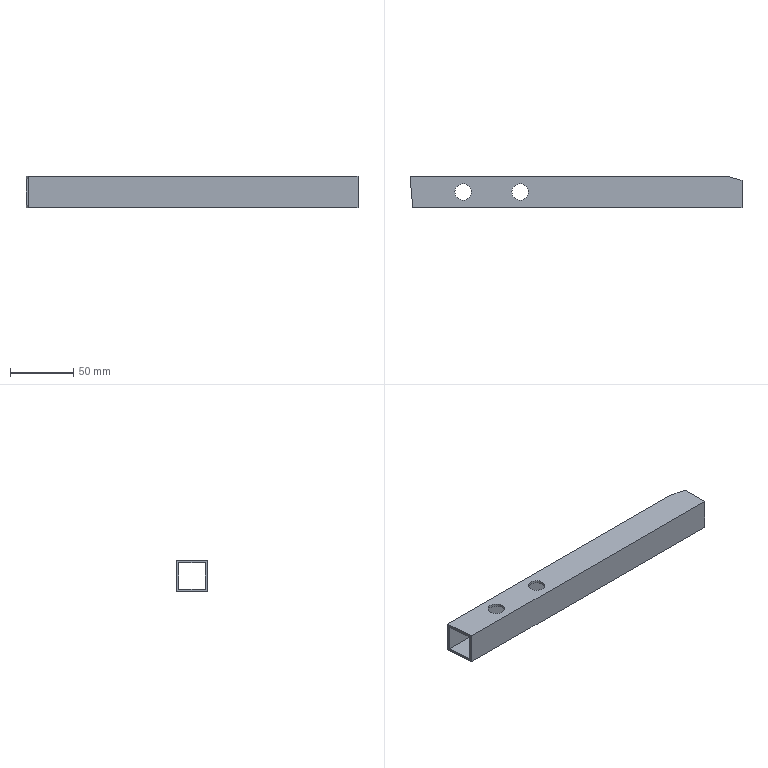Part | NX | features solid 2 | 1 solid | 15 faces | box 261.968 x 25 x 25 mm | volume 46481 mm3 | plane 11 | cylinder 4 | commonest cylinder face diameters 13 x4
STEP:
#1=CARTESIAN_POINT('',(636.5,-100.,-30.));
#2=VERTEX_POINT('',#1);
#3=CARTESIAN_POINT('',(630.,-100.,-30.));
#4=DIRECTION('',(0.,0.,1.));
#5=DIRECTION('',(1.,0.,0.));
#6=AXIS2_PLACEMENT_3D('',#3,#4,#5);
#7=CIRCLE('',#6,6.5);
#8=EDGE_CURVE('',#2,#2,#7,.T.);
#9=ORIENTED_EDGE('',*,*,#8,.F.);
#10=EDGE_LOOP('',(#9));
#11=FACE_BOUND('',#10,.T.);
#12=CARTESIAN_POINT('',(850.,-90.878,-30.));
#13=VERTEX_POINT('',#12);
#14=CARTESIAN_POINT('',(837.392,-87.5,-30.));
#15=VERTEX_POINT('',#14);
#16=CARTESIAN_POINT('',(699.873,-50.652,-30.));
#17=DIRECTION('',(0.9659,-0.2588,0.));
#18=VECTOR('',#17,1000.);
#19=LINE('',#16,#18);
#20=EDGE_CURVE('',#13,#15,#19,.F.);
#21=ORIENTED_EDGE('',*,*,#20,.T.);
#22=CARTESIAN_POINT('',(588.032,-87.5,-30.));
#23=VERTEX_POINT('',#22);
#24=CARTESIAN_POINT('',(690.,-87.5,-30.));
#25=DIRECTION('',(1.,0.,0.));
#26=VECTOR('',#25,1000.);
#27=LINE('',#24,#26);
#28=EDGE_CURVE('',#15,#23,#27,.F.);
#29=ORIENTED_EDGE('',*,*,#28,.T.);
#30=CARTESIAN_POINT('',(590.219,-112.5,-30.));
#31=VERTEX_POINT('',#30);
#32=CARTESIAN_POINT('',(588.806,-96.353,-30.));
#33=DIRECTION('',(-0.08716,0.9962,0.));
#34=VECTOR('',#33,1000.);
#35=LINE('',#32,#34);
#36=EDGE_CURVE('',#23,#31,#35,.F.);
#37=ORIENTED_EDGE('',*,*,#36,.T.);
#38=CARTESIAN_POINT('',(850.,-112.5,-30.));
#39=VERTEX_POINT('',#38);
#40=CARTESIAN_POINT('',(690.,-112.5,-30.));
#41=DIRECTION('',(1.,0.,0.));
#42=VECTOR('',#41,1000.);
#43=LINE('',#40,#42);
#44=EDGE_CURVE('',#39,#31,#43,.F.);
#45=ORIENTED_EDGE('',*,*,#44,.F.);
#46=CARTESIAN_POINT('',(850.,-87.5,-30.));
#47=DIRECTION('',(0.,1.,0.));
#48=VECTOR('',#47,1000.);
#49=LINE('',#46,#48);
#50=EDGE_CURVE('',#13,#39,#49,.F.);
#51=ORIENTED_EDGE('',*,*,#50,.F.);
#52=EDGE_LOOP('',(#21,#29,#37,#45,#51));
#53=FACE_BOUND('',#52,.T.);
#54=CARTESIAN_POINT('',(681.5,-100.,-30.));
#55=VERTEX_POINT('',#54);
#56=CARTESIAN_POINT('',(675.,-100.,-30.));
#57=DIRECTION('',(0.,0.,1.));
#58=DIRECTION('',(1.,0.,0.));
#59=AXIS2_PLACEMENT_3D('',#56,#57,#58);
#60=CIRCLE('',#59,6.5);
#61=EDGE_CURVE('',#55,#55,#60,.F.);
#62=ORIENTED_EDGE('',*,*,#61,.T.);
#63=EDGE_LOOP('',(#62));
#64=FACE_BOUND('',#63,.T.);
#65=CARTESIAN_POINT('',(690.,-87.5,-30.));
#66=DIRECTION('',(0.,0.,-1.));
#67=DIRECTION('',(1.,0.,0.));
#68=AXIS2_PLACEMENT_3D('',#65,#66,#67);
#69=PLANE('',#68);
#70=ADVANCED_FACE('',(#11,#53,#64),#69,.F.);
#71=CARTESIAN_POINT('',(636.5,-100.,-55.));
#72=VERTEX_POINT('',#71);
#73=CARTESIAN_POINT('',(630.,-100.,-55.));
#74=DIRECTION('',(0.,0.,1.));
#75=DIRECTION('',(1.,0.,0.));
#76=AXIS2_PLACEMENT_3D('',#73,#74,#75);
#77=CIRCLE('',#76,6.5);
#78=EDGE_CURVE('',#72,#72,#77,.T.);
#79=ORIENTED_EDGE('',*,*,#78,.T.);
#80=EDGE_LOOP('',(#79));
#81=FACE_BOUND('',#80,.T.);
#82=CARTESIAN_POINT('',(850.,-90.878,-55.));
#83=VERTEX_POINT('',#82);
#84=CARTESIAN_POINT('',(850.,-112.5,-55.));
#85=VERTEX_POINT('',#84);
#86=CARTESIAN_POINT('',(850.,-87.5,-55.));
#87=DIRECTION('',(0.,1.,0.));
#88=VECTOR('',#87,1000.);
#89=LINE('',#86,#88);
#90=EDGE_CURVE('',#83,#85,#89,.F.);
#91=ORIENTED_EDGE('',*,*,#90,.T.);
#92=CARTESIAN_POINT('',(590.219,-112.5,-55.));
#93=VERTEX_POINT('',#92);
#94=CARTESIAN_POINT('',(690.,-112.5,-55.));
#95=DIRECTION('',(-1.,0.,0.));
#96=VECTOR('',#95,1000.);
#97=LINE('',#94,#96);
#98=EDGE_CURVE('',#85,#93,#97,.T.);
#99=ORIENTED_EDGE('',*,*,#98,.T.);
#100=CARTESIAN_POINT('',(588.032,-87.5,-55.));
#101=VERTEX_POINT('',#100);
#102=CARTESIAN_POINT('',(588.806,-96.353,-55.));
#103=DIRECTION('',(-0.08716,0.9962,0.));
#104=VECTOR('',#103,1000.);
#105=LINE('',#102,#104);
#106=EDGE_CURVE('',#101,#93,#105,.F.);
#107=ORIENTED_EDGE('',*,*,#106,.F.);
#108=CARTESIAN_POINT('',(837.392,-87.5,-55.));
#109=VERTEX_POINT('',#108);
#110=CARTESIAN_POINT('',(690.,-87.5,-55.));
#111=DIRECTION('',(-1.,0.,0.));
#112=VECTOR('',#111,1000.);
#113=LINE('',#110,#112);
#114=EDGE_CURVE('',#109,#101,#113,.T.);
#115=ORIENTED_EDGE('',*,*,#114,.F.);
#116=CARTESIAN_POINT('',(699.873,-50.652,-55.));
#117=DIRECTION('',(0.9659,-0.2588,0.));
#118=VECTOR('',#117,1000.);
#119=LINE('',#116,#118);
#120=EDGE_CURVE('',#83,#109,#119,.F.);
#121=ORIENTED_EDGE('',*,*,#120,.F.);
#122=EDGE_LOOP('',(#91,#99,#107,#115,#121));
#123=FACE_BOUND('',#122,.T.);
#124=CARTESIAN_POINT('',(681.5,-100.,-55.));
#125=VERTEX_POINT('',#124);
#126=CARTESIAN_POINT('',(675.,-100.,-55.));
#127=DIRECTION('',(0.,0.,1.));
#128=DIRECTION('',(1.,0.,0.));
#129=AXIS2_PLACEMENT_3D('',#126,#127,#128);
#130=CIRCLE('',#129,6.5);
#131=EDGE_CURVE('',#125,#125,#130,.F.);
#132=ORIENTED_EDGE('',*,*,#131,.F.);
#133=EDGE_LOOP('',(#132));
#134=FACE_BOUND('',#133,.T.);
#135=CARTESIAN_POINT('',(690.,-87.5,-55.));
#136=DIRECTION('',(0.,0.,-1.));
#137=DIRECTION('',(1.,0.,0.));
#138=AXIS2_PLACEMENT_3D('',#135,#136,#137);
#139=PLANE('',#138);
#140=ADVANCED_FACE('',(#81,#123,#134),#139,.T.);
#141=CARTESIAN_POINT('',(636.5,-100.,-32.));
#142=VERTEX_POINT('',#141);
#143=CARTESIAN_POINT('',(630.,-100.,-32.));
#144=DIRECTION('',(0.,0.,1.));
#145=DIRECTION('',(1.,0.,0.));
#146=AXIS2_PLACEMENT_3D('',#143,#144,#145);
#147=CIRCLE('',#146,6.5);
#148=EDGE_CURVE('',#142,#142,#147,.T.);
#149=ORIENTED_EDGE('',*,*,#148,.T.);
#150=EDGE_LOOP('',(#149));
#151=FACE_BOUND('',#150,.T.);
#152=CARTESIAN_POINT('',(850.,-90.878,-32.));
#153=VERTEX_POINT('',#152);
#154=CARTESIAN_POINT('',(850.,-110.5,-32.));
#155=VERTEX_POINT('',#154);
#156=CARTESIAN_POINT('',(850.,-87.5,-32.));
#157=DIRECTION('',(0.,1.,0.));
#158=VECTOR('',#157,1000.);
#159=LINE('',#156,#158);
#160=EDGE_CURVE('',#153,#155,#159,.F.);
#161=ORIENTED_EDGE('',*,*,#160,.T.);
#162=CARTESIAN_POINT('',(590.044,-110.5,-32.));
#163=VERTEX_POINT('',#162);
#164=CARTESIAN_POINT('',(690.,-110.5,-32.));
#165=DIRECTION('',(1.,0.,0.));
#166=VECTOR('',#165,1000.);
#167=LINE('',#164,#166);
#168=EDGE_CURVE('',#155,#163,#167,.F.);
#169=ORIENTED_EDGE('',*,*,#168,.T.);
#170=CARTESIAN_POINT('',(588.206,-89.5,-32.));
#171=VERTEX_POINT('',#170);
#172=CARTESIAN_POINT('',(587.821,-85.095,-32.));
#173=DIRECTION('',(0.08716,-0.9962,0.));
#174=VECTOR('',#173,1000.);
#175=LINE('',#172,#174);
#176=EDGE_CURVE('',#163,#171,#175,.F.);
#177=ORIENTED_EDGE('',*,*,#176,.T.);
#178=CARTESIAN_POINT('',(844.856,-89.5,-32.));
#179=VERTEX_POINT('',#178);
#180=CARTESIAN_POINT('',(690.,-89.5,-32.));
#181=DIRECTION('',(-1.,0.,0.));
#182=VECTOR('',#181,1000.);
#183=LINE('',#180,#182);
#184=EDGE_CURVE('',#179,#171,#183,.T.);
#185=ORIENTED_EDGE('',*,*,#184,.F.);
#186=CARTESIAN_POINT('',(699.873,-50.652,-32.));
#187=DIRECTION('',(0.9659,-0.2588,0.));
#188=VECTOR('',#187,1000.);
#189=LINE('',#186,#188);
#190=EDGE_CURVE('',#153,#179,#189,.F.);
#191=ORIENTED_EDGE('',*,*,#190,.F.);
#192=EDGE_LOOP('',(#161,#169,#177,#185,#191));
#193=FACE_BOUND('',#192,.T.);
#194=CARTESIAN_POINT('',(681.5,-100.,-32.));
#195=VERTEX_POINT('',#194);
#196=CARTESIAN_POINT('',(675.,-100.,-32.));
#197=DIRECTION('',(0.,0.,1.));
#198=DIRECTION('',(1.,0.,0.));
#199=AXIS2_PLACEMENT_3D('',#196,#197,#198);
#200=CIRCLE('',#199,6.5);
#201=EDGE_CURVE('',#195,#195,#200,.F.);
#202=ORIENTED_EDGE('',*,*,#201,.F.);
#203=EDGE_LOOP('',(#202));
#204=FACE_BOUND('',#203,.T.);
#205=CARTESIAN_POINT('',(690.,-87.5,-32.));
#206=DIRECTION('',(0.,0.,-1.));
#207=DIRECTION('',(1.,0.,0.));
#208=AXIS2_PLACEMENT_3D('',#205,#206,#207);
#209=PLANE('',#208);
#210=ADVANCED_FACE('',(#151,#193,#204),#209,.T.);
#211=CARTESIAN_POINT('',(636.5,-100.,-53.));
#212=VERTEX_POINT('',#211);
#213=CARTESIAN_POINT('',(630.,-100.,-53.));
#214=DIRECTION('',(0.,0.,1.));
#215=DIRECTION('',(1.,0.,0.));
#216=AXIS2_PLACEMENT_3D('',#213,#214,#215);
#217=CIRCLE('',#216,6.5);
#218=EDGE_CURVE('',#212,#212,#217,.T.);
#219=ORIENTED_EDGE('',*,*,#218,.F.);
#220=EDGE_LOOP('',(#219));
#221=FACE_BOUND('',#220,.T.);
#222=CARTESIAN_POINT('',(850.,-90.878,-53.));
#223=VERTEX_POINT('',#222);
#224=CARTESIAN_POINT('',(844.856,-89.5,-53.));
#225=VERTEX_POINT('',#224);
#226=CARTESIAN_POINT('',(699.873,-50.652,-53.));
#227=DIRECTION('',(0.9659,-0.2588,0.));
#228=VECTOR('',#227,1000.);
#229=LINE('',#226,#228);
#230=EDGE_CURVE('',#223,#225,#229,.F.);
#231=ORIENTED_EDGE('',*,*,#230,.T.);
#232=CARTESIAN_POINT('',(588.206,-89.5,-53.));
#233=VERTEX_POINT('',#232);
#234=CARTESIAN_POINT('',(690.,-89.5,-53.));
#235=DIRECTION('',(-1.,0.,0.));
#236=VECTOR('',#235,1000.);
#237=LINE('',#234,#236);
#238=EDGE_CURVE('',#225,#233,#237,.T.);
#239=ORIENTED_EDGE('',*,*,#238,.T.);
#240=CARTESIAN_POINT('',(590.044,-110.5,-53.));
#241=VERTEX_POINT('',#240);
#242=CARTESIAN_POINT('',(587.821,-85.095,-53.));
#243=DIRECTION('',(0.08716,-0.9962,0.));
#244=VECTOR('',#243,1000.);
#245=LINE('',#242,#244);
#246=EDGE_CURVE('',#241,#233,#245,.F.);
#247=ORIENTED_EDGE('',*,*,#246,.F.);
#248=CARTESIAN_POINT('',(850.,-110.5,-53.));
#249=VERTEX_POINT('',#248);
#250=CARTESIAN_POINT('',(690.,-110.5,-53.));
#251=DIRECTION('',(1.,0.,0.));
#252=VECTOR('',#251,1000.);
#253=LINE('',#250,#252);
#254=EDGE_CURVE('',#249,#241,#253,.F.);
#255=ORIENTED_EDGE('',*,*,#254,.F.);
#256=CARTESIAN_POINT('',(850.,-87.5,-53.));
#257=DIRECTION('',(0.,1.,0.));
#258=VECTOR('',#257,1000.);
#259=LINE('',#256,#258);
#260=EDGE_CURVE('',#223,#249,#259,.F.);
#261=ORIENTED_EDGE('',*,*,#260,.F.);
#262=EDGE_LOOP('',(#231,#239,#247,#255,#261));
#263=FACE_BOUND('',#262,.T.);
#264=CARTESIAN_POINT('',(681.5,-100.,-53.));
#265=VERTEX_POINT('',#264);
#266=CARTESIAN_POINT('',(675.,-100.,-53.));
#267=DIRECTION('',(0.,0.,1.));
#268=DIRECTION('',(1.,0.,0.));
#269=AXIS2_PLACEMENT_3D('',#266,#267,#268);
#270=CIRCLE('',#269,6.5);
#271=EDGE_CURVE('',#265,#265,#270,.F.);
#272=ORIENTED_EDGE('',*,*,#271,.T.);
#273=EDGE_LOOP('',(#272));
#274=FACE_BOUND('',#273,.T.);
#275=CARTESIAN_POINT('',(690.,-87.5,-53.));
#276=DIRECTION('',(0.,0.,-1.));
#277=DIRECTION('',(1.,0.,0.));
#278=AXIS2_PLACEMENT_3D('',#275,#276,#277);
#279=PLANE('',#278);
#280=ADVANCED_FACE('',(#221,#263,#274),#279,.F.);
#281=ORIENTED_EDGE('',*,*,#50,.T.);
#282=CARTESIAN_POINT('',(850.,-112.5,-55.));
#283=DIRECTION('',(0.,0.,1.));
#284=VECTOR('',#283,1000.);
#285=LINE('',#282,#284);
#286=EDGE_CURVE('',#85,#39,#285,.T.);
#287=ORIENTED_EDGE('',*,*,#286,.F.);
#288=ORIENTED_EDGE('',*,*,#90,.F.);
#289=CARTESIAN_POINT('',(850.,-90.878,-55.));
#290=DIRECTION('',(0.,0.,-1.));
#291=VECTOR('',#290,1000.);
#292=LINE('',#289,#291);
#293=EDGE_CURVE('',#223,#83,#292,.T.);
#294=ORIENTED_EDGE('',*,*,#293,.F.);
#295=ORIENTED_EDGE('',*,*,#260,.T.);
#296=CARTESIAN_POINT('',(850.,-110.5,-55.));
#297=DIRECTION('',(0.,0.,1.));
#298=VECTOR('',#297,1000.);
#299=LINE('',#296,#298);
#300=EDGE_CURVE('',#249,#155,#299,.T.);
#301=ORIENTED_EDGE('',*,*,#300,.T.);
#302=ORIENTED_EDGE('',*,*,#160,.F.);
#303=CARTESIAN_POINT('',(850.,-90.878,-55.));
#304=DIRECTION('',(0.,0.,-1.));
#305=VECTOR('',#304,1000.);
#306=LINE('',#303,#305);
#307=EDGE_CURVE('',#13,#153,#306,.T.);
#308=ORIENTED_EDGE('',*,*,#307,.F.);
#309=EDGE_LOOP('',(#281,#287,#288,#294,#295,#301,#302,#308));
#310=FACE_BOUND('',#309,.T.);
#311=CARTESIAN_POINT('',(850.,-87.5,-55.));
#312=DIRECTION('',(-1.,0.,0.));
#313=DIRECTION('',(0.,-1.,0.));
#314=AXIS2_PLACEMENT_3D('',#311,#312,#313);
#315=PLANE('',#314);
#316=ADVANCED_FACE('',(#310),#315,.F.);
#317=ORIENTED_EDGE('',*,*,#114,.T.);
#318=CARTESIAN_POINT('',(588.032,-87.5,-30.));
#319=DIRECTION('',(0.,0.,-1.));
#320=VECTOR('',#319,1000.);
#321=LINE('',#318,#320);
#322=EDGE_CURVE('',#101,#23,#321,.F.);
#323=ORIENTED_EDGE('',*,*,#322,.T.);
#324=ORIENTED_EDGE('',*,*,#28,.F.);
#325=CARTESIAN_POINT('',(837.392,-87.5,-55.));
#326=DIRECTION('',(0.,0.,-1.));
#327=VECTOR('',#326,1000.);
#328=LINE('',#325,#327);
#329=EDGE_CURVE('',#109,#15,#328,.F.);
#330=ORIENTED_EDGE('',*,*,#329,.F.);
#331=EDGE_LOOP('',(#317,#323,#324,#330));
#332=FACE_BOUND('',#331,.T.);
#333=CARTESIAN_POINT('',(690.,-87.5,-55.));
#334=DIRECTION('',(0.,1.,0.));
#335=DIRECTION('',(-1.,0.,0.));
#336=AXIS2_PLACEMENT_3D('',#333,#334,#335);
#337=PLANE('',#336);
#338=ADVANCED_FACE('',(#332),#337,.T.);
#339=CARTESIAN_POINT('',(844.856,-89.5,-55.));
#340=DIRECTION('',(0.,0.,-1.));
#341=VECTOR('',#340,1000.);
#342=LINE('',#339,#341);
#343=EDGE_CURVE('',#225,#179,#342,.F.);
#344=ORIENTED_EDGE('',*,*,#343,.T.);
#345=ORIENTED_EDGE('',*,*,#184,.T.);
#346=CARTESIAN_POINT('',(588.206,-89.5,-55.));
#347=DIRECTION('',(0.,0.,1.));
#348=VECTOR('',#347,1000.);
#349=LINE('',#346,#348);
#350=EDGE_CURVE('',#171,#233,#349,.F.);
#351=ORIENTED_EDGE('',*,*,#350,.T.);
#352=ORIENTED_EDGE('',*,*,#238,.F.);
#353=EDGE_LOOP('',(#344,#345,#351,#352));
#354=FACE_BOUND('',#353,.T.);
#355=CARTESIAN_POINT('',(690.,-89.5,-55.));
#356=DIRECTION('',(0.,1.,0.));
#357=DIRECTION('',(-1.,0.,0.));
#358=AXIS2_PLACEMENT_3D('',#355,#356,#357);
#359=PLANE('',#358);
#360=ADVANCED_FACE('',(#354),#359,.F.);
#361=ORIENTED_EDGE('',*,*,#286,.T.);
#362=ORIENTED_EDGE('',*,*,#44,.T.);
#363=CARTESIAN_POINT('',(590.219,-112.5,-55.));
#364=DIRECTION('',(0.,0.,1.));
#365=VECTOR('',#364,1000.);
#366=LINE('',#363,#365);
#367=EDGE_CURVE('',#93,#31,#366,.T.);
#368=ORIENTED_EDGE('',*,*,#367,.F.);
#369=ORIENTED_EDGE('',*,*,#98,.F.);
#370=EDGE_LOOP('',(#361,#362,#368,#369));
#371=FACE_BOUND('',#370,.T.);
#372=CARTESIAN_POINT('',(690.,-112.5,-55.));
#373=DIRECTION('',(0.,1.,0.));
#374=DIRECTION('',(-1.,0.,0.));
#375=AXIS2_PLACEMENT_3D('',#372,#373,#374);
#376=PLANE('',#375);
#377=ADVANCED_FACE('',(#371),#376,.F.);
#378=ORIENTED_EDGE('',*,*,#246,.T.);
#379=ORIENTED_EDGE('',*,*,#350,.F.);
#380=ORIENTED_EDGE('',*,*,#176,.F.);
#381=CARTESIAN_POINT('',(590.044,-110.5,-30.));
#382=DIRECTION('',(0.,0.,-1.));
#383=VECTOR('',#382,1000.);
#384=LINE('',#381,#383);
#385=EDGE_CURVE('',#163,#241,#384,.T.);
#386=ORIENTED_EDGE('',*,*,#385,.T.);
#387=EDGE_LOOP('',(#378,#379,#380,#386));
#388=FACE_BOUND('',#387,.T.);
#389=ORIENTED_EDGE('',*,*,#106,.T.);
#390=ORIENTED_EDGE('',*,*,#367,.T.);
#391=ORIENTED_EDGE('',*,*,#36,.F.);
#392=ORIENTED_EDGE('',*,*,#322,.F.);
#393=EDGE_LOOP('',(#389,#390,#391,#392));
#394=FACE_BOUND('',#393,.T.);
#395=CARTESIAN_POINT('',(587.821,-85.095,-30.));
#396=DIRECTION('',(0.9962,0.08716,0.));
#397=DIRECTION('',(0.,0.,1.));
#398=AXIS2_PLACEMENT_3D('',#395,#396,#397);
#399=PLANE('',#398);
#400=ADVANCED_FACE('',(#388,#394),#399,.F.);
#401=ORIENTED_EDGE('',*,*,#385,.F.);
#402=ORIENTED_EDGE('',*,*,#168,.F.);
#403=ORIENTED_EDGE('',*,*,#300,.F.);
#404=ORIENTED_EDGE('',*,*,#254,.T.);
#405=EDGE_LOOP('',(#401,#402,#403,#404));
#406=FACE_BOUND('',#405,.T.);
#407=CARTESIAN_POINT('',(690.,-110.5,-55.));
#408=DIRECTION('',(0.,1.,0.));
#409=DIRECTION('',(-1.,0.,0.));
#410=AXIS2_PLACEMENT_3D('',#407,#408,#409);
#411=PLANE('',#410);
#412=ADVANCED_FACE('',(#406),#411,.T.);
#413=ORIENTED_EDGE('',*,*,#307,.T.);
#414=ORIENTED_EDGE('',*,*,#190,.T.);
#415=ORIENTED_EDGE('',*,*,#343,.F.);
#416=ORIENTED_EDGE('',*,*,#230,.F.);
#417=ORIENTED_EDGE('',*,*,#293,.T.);
#418=ORIENTED_EDGE('',*,*,#120,.T.);
#419=ORIENTED_EDGE('',*,*,#329,.T.);
#420=ORIENTED_EDGE('',*,*,#20,.F.);
#421=EDGE_LOOP('',(#413,#414,#415,#416,#417,#418,#419,#420));
#422=FACE_BOUND('',#421,.T.);
#423=CARTESIAN_POINT('',(839.148,-87.97,-30.));
#424=DIRECTION('',(-0.2588,-0.9659,0.));
#425=DIRECTION('',(0.,0.,1.));
#426=AXIS2_PLACEMENT_3D('',#423,#424,#425);
#427=PLANE('',#426);
#428=ADVANCED_FACE('',(#422),#427,.F.);
#429=ORIENTED_EDGE('',*,*,#131,.T.);
#430=EDGE_LOOP('',(#429));
#431=FACE_BOUND('',#430,.T.);
#432=ORIENTED_EDGE('',*,*,#271,.F.);
#433=EDGE_LOOP('',(#432));
#434=FACE_BOUND('',#433,.T.);
#435=CARTESIAN_POINT('',(675.,-100.,-255.));
#436=DIRECTION('',(0.,0.,1.));
#437=DIRECTION('',(-1.,0.,0.));
#438=AXIS2_PLACEMENT_3D('',#435,#436,#437);
#439=CYLINDRICAL_SURFACE('',#438,6.5);
#440=ADVANCED_FACE('',(#431,#434),#439,.F.);
#441=ORIENTED_EDGE('',*,*,#201,.T.);
#442=EDGE_LOOP('',(#441));
#443=FACE_BOUND('',#442,.T.);
#444=ORIENTED_EDGE('',*,*,#61,.F.);
#445=EDGE_LOOP('',(#444));
#446=FACE_BOUND('',#445,.T.);
#447=CARTESIAN_POINT('',(675.,-100.,-255.));
#448=DIRECTION('',(0.,0.,1.));
#449=DIRECTION('',(-1.,0.,0.));
#450=AXIS2_PLACEMENT_3D('',#447,#448,#449);
#451=CYLINDRICAL_SURFACE('',#450,6.5);
#452=ADVANCED_FACE('',(#443,#446),#451,.F.);
#453=ORIENTED_EDGE('',*,*,#78,.F.);
#454=EDGE_LOOP('',(#453));
#455=FACE_BOUND('',#454,.T.);
#456=ORIENTED_EDGE('',*,*,#218,.T.);
#457=EDGE_LOOP('',(#456));
#458=FACE_BOUND('',#457,.T.);
#459=CARTESIAN_POINT('',(630.,-100.,-255.));
#460=DIRECTION('',(0.,0.,1.));
#461=DIRECTION('',(-1.,0.,0.));
#462=AXIS2_PLACEMENT_3D('',#459,#460,#461);
#463=CYLINDRICAL_SURFACE('',#462,6.5);
#464=ADVANCED_FACE('',(#455,#458),#463,.F.);
#465=ORIENTED_EDGE('',*,*,#148,.F.);
#466=EDGE_LOOP('',(#465));
#467=FACE_BOUND('',#466,.T.);
#468=ORIENTED_EDGE('',*,*,#8,.T.);
#469=EDGE_LOOP('',(#468));
#470=FACE_BOUND('',#469,.T.);
#471=CARTESIAN_POINT('',(630.,-100.,-255.));
#472=DIRECTION('',(0.,0.,1.));
#473=DIRECTION('',(-1.,0.,0.));
#474=AXIS2_PLACEMENT_3D('',#471,#472,#473);
#475=CYLINDRICAL_SURFACE('',#474,6.5);
#476=ADVANCED_FACE('',(#467,#470),#475,.F.);
#477=CLOSED_SHELL('',(#70,#140,#210,#280,#316,#338,#360,#377,#400,#412,#428,#440,#452,#464,#476));
#478=MANIFOLD_SOLID_BREP('',#477);
#479=(LENGTH_UNIT()NAMED_UNIT(*)SI_UNIT(.MILLI.,.METRE.));
#480=UNCERTAINTY_MEASURE_WITH_UNIT(LENGTH_MEASURE(0.00001),#479,'','');
#481=(NAMED_UNIT(*)PLANE_ANGLE_UNIT()SI_UNIT($,.RADIAN.));
#482=(NAMED_UNIT(*)SI_UNIT($,.STERADIAN.)SOLID_ANGLE_UNIT());
#483=(GEOMETRIC_REPRESENTATION_CONTEXT(3)GLOBAL_UNCERTAINTY_ASSIGNED_CONTEXT((#480))GLOBAL_UNIT_ASSIGNED_CONTEXT((#479,#481,#482))REPRESENTATION_CONTEXT('',''));
#484=ADVANCED_BREP_SHAPE_REPRESENTATION('',(#478),#483);